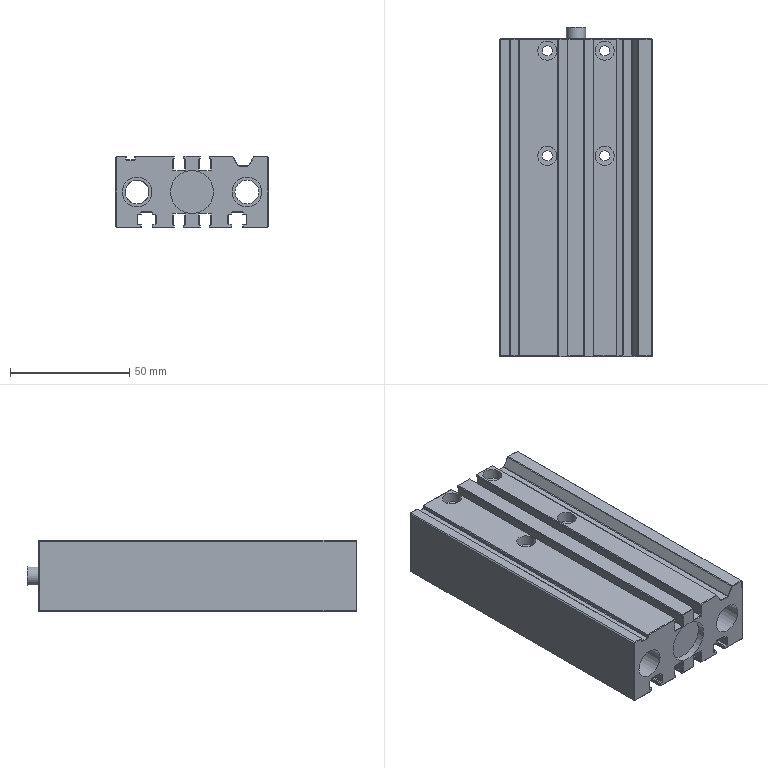Part | STEP file | Tube feed_id890_x_t | 1 solid | 430 faces | box 64 x 137.8 x 30 mm | volume 193206 mm3 | plane 413 | cylinder 17 | commonest cylinder face diameters 8 x5 4.2 x4 15 x3 10 x2 12.5 x2 18 x1